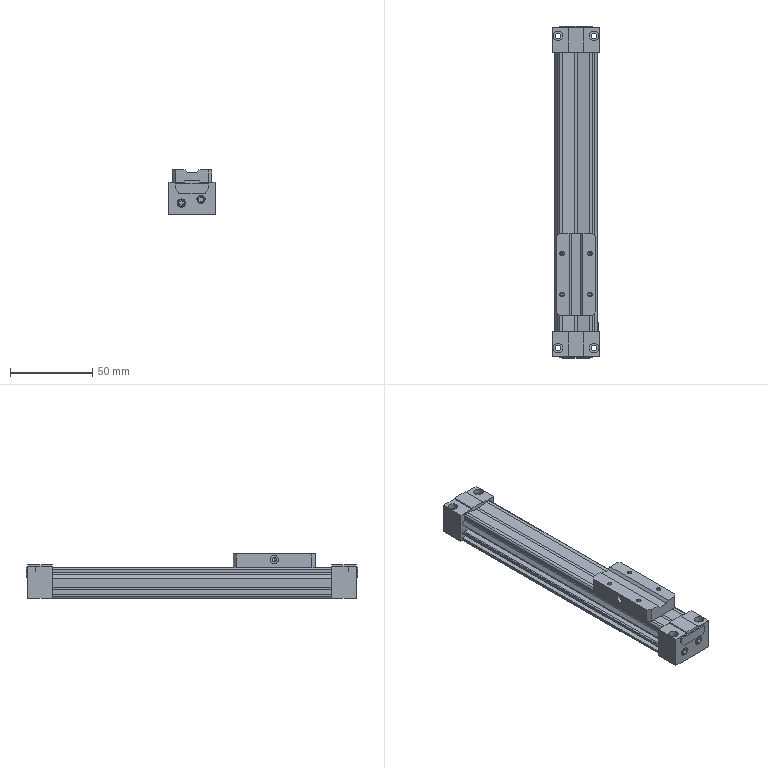Part | SolidWorks | 7 solids | 330 faces | box 28 x 202 x 27 mm | volume 86824 mm3 | plane 195 | cylinder 91 | cone 32 | torus 12 | commonest cylinder face diameters 5 x20 2.459 x12 4 x11 3.4 x8 4.4 x8 5.8 x8